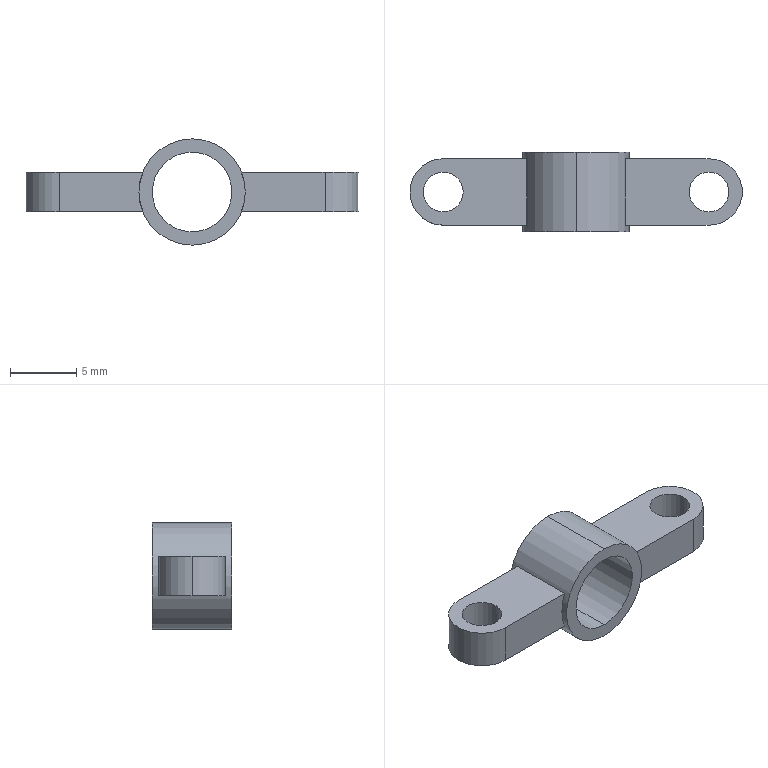Part | SolidWorks | features Extrusion 1, ICE 1 | 1 solid | 21 faces | box 25 x 6 x 8 mm | volume 331.315 mm3 | cylinder 11 | plane 10 | commonest cylinder face diameters 3 x4 5 x3 6 x2 8 x2
STEP:
#1=CARTESIAN_POINT('',(-11.5,3.,1.5));
#2=VERTEX_POINT('',#1);
#3=CARTESIAN_POINT('',(-8.5,3.,1.5));
#4=VERTEX_POINT('',#3);
#5=CARTESIAN_POINT('',(-10.,3.,1.5));
#6=DIRECTION('',(0.,0.,1.));
#7=DIRECTION('',(1.,0.,0.));
#8=AXIS2_PLACEMENT_3D('',#5,#6,#7);
#9=CIRCLE('',#8,1.5);
#10=EDGE_CURVE('',#2,#4,#9,.T.);
#11=ORIENTED_EDGE('',*,*,#10,.T.);
#12=CARTESIAN_POINT('',(-8.5,3.,-1.5));
#13=VERTEX_POINT('',#12);
#14=CARTESIAN_POINT('',(-8.5,3.,1.5));
#15=DIRECTION('',(0.,0.,-1.));
#16=VECTOR('',#15,1000.);
#17=LINE('',#14,#16);
#18=EDGE_CURVE('',#4,#13,#17,.T.);
#19=ORIENTED_EDGE('',*,*,#18,.T.);
#20=CARTESIAN_POINT('',(-11.5,3.,-1.5));
#21=VERTEX_POINT('',#20);
#22=CARTESIAN_POINT('',(-10.,3.,-1.5));
#23=DIRECTION('',(0.,0.,1.));
#24=DIRECTION('',(1.,0.,0.));
#25=AXIS2_PLACEMENT_3D('',#22,#23,#24);
#26=CIRCLE('',#25,1.5);
#27=EDGE_CURVE('',#21,#13,#26,.T.);
#28=ORIENTED_EDGE('',*,*,#27,.F.);
#29=CARTESIAN_POINT('',(-11.5,3.,1.5));
#30=DIRECTION('',(0.,0.,-1.));
#31=VECTOR('',#30,1000.);
#32=LINE('',#29,#31);
#33=EDGE_CURVE('',#2,#21,#32,.T.);
#34=ORIENTED_EDGE('',*,*,#33,.F.);
#35=EDGE_LOOP('',(#11,#19,#28,#34));
#36=FACE_OUTER_BOUND('',#35,.T.);
#37=CARTESIAN_POINT('',(-10.,3.,1.5));
#38=DIRECTION('',(0.,0.,-1.));
#39=DIRECTION('',(-1.,0.,0.));
#40=AXIS2_PLACEMENT_3D('',#37,#38,#39);
#41=CYLINDRICAL_SURFACE('',#40,1.5);
#42=ADVANCED_FACE('',(#36),#41,.F.);
#43=CARTESIAN_POINT('',(-12.5,3.,1.5));
#44=VERTEX_POINT('',#43);
#45=CARTESIAN_POINT('',(-10.,0.5,1.5));
#46=VERTEX_POINT('',#45);
#47=CARTESIAN_POINT('',(-10.,3.,1.5));
#48=DIRECTION('',(0.,0.,1.));
#49=DIRECTION('',(1.,0.,0.));
#50=AXIS2_PLACEMENT_3D('',#47,#48,#49);
#51=CIRCLE('',#50,2.5);
#52=EDGE_CURVE('',#44,#46,#51,.T.);
#53=ORIENTED_EDGE('',*,*,#52,.F.);
#54=CARTESIAN_POINT('',(-12.5,3.,-1.5));
#55=VERTEX_POINT('',#54);
#56=CARTESIAN_POINT('',(-12.5,3.,1.5));
#57=DIRECTION('',(0.,0.,-1.));
#58=VECTOR('',#57,1000.);
#59=LINE('',#56,#58);
#60=EDGE_CURVE('',#44,#55,#59,.T.);
#61=ORIENTED_EDGE('',*,*,#60,.T.);
#62=CARTESIAN_POINT('',(-10.,0.5,-1.5));
#63=VERTEX_POINT('',#62);
#64=CARTESIAN_POINT('',(-10.,3.,-1.5));
#65=DIRECTION('',(0.,0.,1.));
#66=DIRECTION('',(1.,0.,0.));
#67=AXIS2_PLACEMENT_3D('',#64,#65,#66);
#68=CIRCLE('',#67,2.5);
#69=EDGE_CURVE('',#55,#63,#68,.T.);
#70=ORIENTED_EDGE('',*,*,#69,.T.);
#71=CARTESIAN_POINT('',(-10.,0.5,1.5));
#72=DIRECTION('',(0.,0.,-1.));
#73=VECTOR('',#72,1000.);
#74=LINE('',#71,#73);
#75=EDGE_CURVE('',#46,#63,#74,.T.);
#76=ORIENTED_EDGE('',*,*,#75,.F.);
#77=EDGE_LOOP('',(#53,#61,#70,#76));
#78=FACE_OUTER_BOUND('',#77,.T.);
#79=CARTESIAN_POINT('',(-10.,3.,1.5));
#80=DIRECTION('',(0.,0.,-1.));
#81=DIRECTION('',(-1.,0.,0.));
#82=AXIS2_PLACEMENT_3D('',#79,#80,#81);
#83=CYLINDRICAL_SURFACE('',#82,2.5);
#84=ADVANCED_FACE('',(#78),#83,.T.);
#85=CARTESIAN_POINT('',(11.5,3.,1.5));
#86=VERTEX_POINT('',#85);
#87=CARTESIAN_POINT('',(8.5,3.,1.5));
#88=VERTEX_POINT('',#87);
#89=CARTESIAN_POINT('',(10.,3.,1.5));
#90=DIRECTION('',(0.,0.,-1.));
#91=DIRECTION('',(1.,0.,0.));
#92=AXIS2_PLACEMENT_3D('',#89,#90,#91);
#93=CIRCLE('',#92,1.5);
#94=EDGE_CURVE('',#86,#88,#93,.T.);
#95=ORIENTED_EDGE('',*,*,#94,.F.);
#96=CARTESIAN_POINT('',(11.5,3.,-1.5));
#97=VERTEX_POINT('',#96);
#98=CARTESIAN_POINT('',(11.5,3.,1.5));
#99=DIRECTION('',(0.,0.,-1.));
#100=VECTOR('',#99,1000.);
#101=LINE('',#98,#100);
#102=EDGE_CURVE('',#86,#97,#101,.T.);
#103=ORIENTED_EDGE('',*,*,#102,.T.);
#104=CARTESIAN_POINT('',(8.5,3.,-1.5));
#105=VERTEX_POINT('',#104);
#106=CARTESIAN_POINT('',(10.,3.,-1.5));
#107=DIRECTION('',(0.,0.,-1.));
#108=DIRECTION('',(1.,0.,0.));
#109=AXIS2_PLACEMENT_3D('',#106,#107,#108);
#110=CIRCLE('',#109,1.5);
#111=EDGE_CURVE('',#97,#105,#110,.T.);
#112=ORIENTED_EDGE('',*,*,#111,.T.);
#113=CARTESIAN_POINT('',(8.5,3.,1.5));
#114=DIRECTION('',(0.,0.,-1.));
#115=VECTOR('',#114,1000.);
#116=LINE('',#113,#115);
#117=EDGE_CURVE('',#88,#105,#116,.T.);
#118=ORIENTED_EDGE('',*,*,#117,.F.);
#119=EDGE_LOOP('',(#95,#103,#112,#118));
#120=FACE_OUTER_BOUND('',#119,.T.);
#121=CARTESIAN_POINT('',(10.,3.,1.5));
#122=DIRECTION('',(0.,0.,-1.));
#123=DIRECTION('',(-1.,0.,0.));
#124=AXIS2_PLACEMENT_3D('',#121,#122,#123);
#125=CYLINDRICAL_SURFACE('',#124,1.5);
#126=ADVANCED_FACE('',(#120),#125,.F.);
#127=CARTESIAN_POINT('',(0.,6.,-3.));
#128=VERTEX_POINT('',#127);
#129=CARTESIAN_POINT('',(0.,6.,3.));
#130=VERTEX_POINT('',#129);
#131=CARTESIAN_POINT('',(0.,6.,0.));
#132=DIRECTION('',(0.,1.,0.));
#133=DIRECTION('',(0.,0.,1.));
#134=AXIS2_PLACEMENT_3D('',#131,#132,#133);
#135=CIRCLE('',#134,3.);
#136=EDGE_CURVE('',#128,#130,#135,.T.);
#137=ORIENTED_EDGE('',*,*,#136,.T.);
#138=CARTESIAN_POINT('',(0.,0.,3.));
#139=VERTEX_POINT('',#138);
#140=CARTESIAN_POINT('',(0.,6.,3.));
#141=DIRECTION('',(0.,-1.,0.));
#142=VECTOR('',#141,1000.);
#143=LINE('',#140,#142);
#144=EDGE_CURVE('',#130,#139,#143,.T.);
#145=ORIENTED_EDGE('',*,*,#144,.T.);
#146=CARTESIAN_POINT('',(0.,0.,-3.));
#147=VERTEX_POINT('',#146);
#148=CARTESIAN_POINT('',(0.,0.,0.));
#149=DIRECTION('',(0.,1.,0.));
#150=DIRECTION('',(0.,0.,1.));
#151=AXIS2_PLACEMENT_3D('',#148,#149,#150);
#152=CIRCLE('',#151,3.);
#153=EDGE_CURVE('',#147,#139,#152,.T.);
#154=ORIENTED_EDGE('',*,*,#153,.F.);
#155=CARTESIAN_POINT('',(0.,6.,-3.));
#156=DIRECTION('',(0.,-1.,0.));
#157=VECTOR('',#156,1000.);
#158=LINE('',#155,#157);
#159=EDGE_CURVE('',#128,#147,#158,.T.);
#160=ORIENTED_EDGE('',*,*,#159,.F.);
#161=EDGE_LOOP('',(#137,#145,#154,#160));
#162=FACE_OUTER_BOUND('',#161,.T.);
#163=CARTESIAN_POINT('',(0.,6.,0.));
#164=DIRECTION('',(0.,-1.,0.));
#165=DIRECTION('',(0.,0.,-1.));
#166=AXIS2_PLACEMENT_3D('',#163,#164,#165);
#167=CYLINDRICAL_SURFACE('',#166,3.);
#168=ADVANCED_FACE('',(#162),#167,.F.);
#169=CARTESIAN_POINT('',(3.708,0.5,1.5));
#170=VERTEX_POINT('',#169);
#171=CARTESIAN_POINT('',(3.708,0.5,-1.5));
#172=VERTEX_POINT('',#171);
#173=CARTESIAN_POINT('',(0.,0.5,0.));
#174=DIRECTION('',(0.,1.,0.));
#175=DIRECTION('',(-1.,0.,0.));
#176=AXIS2_PLACEMENT_3D('',#173,#174,#175);
#177=CIRCLE('',#176,4.);
#178=EDGE_CURVE('',#170,#172,#177,.T.);
#179=ORIENTED_EDGE('',*,*,#178,.F.);
#180=CARTESIAN_POINT('',(3.708,5.5,1.5));
#181=VERTEX_POINT('',#180);
#182=CARTESIAN_POINT('',(3.708,6.,1.5));
#183=DIRECTION('',(0.,1.,0.));
#184=VECTOR('',#183,1000.);
#185=LINE('',#182,#184);
#186=EDGE_CURVE('',#170,#181,#185,.T.);
#187=ORIENTED_EDGE('',*,*,#186,.T.);
#188=CARTESIAN_POINT('',(3.708,5.5,-1.5));
#189=VERTEX_POINT('',#188);
#190=CARTESIAN_POINT('',(0.,5.5,0.));
#191=DIRECTION('',(0.,-1.,0.));
#192=DIRECTION('',(0.,0.,-1.));
#193=AXIS2_PLACEMENT_3D('',#190,#191,#192);
#194=CIRCLE('',#193,4.);
#195=EDGE_CURVE('',#189,#181,#194,.T.);
#196=ORIENTED_EDGE('',*,*,#195,.F.);
#197=CARTESIAN_POINT('',(3.708,6.,-1.5));
#198=DIRECTION('',(0.,1.,0.));
#199=VECTOR('',#198,1000.);
#200=LINE('',#197,#199);
#201=EDGE_CURVE('',#172,#189,#200,.T.);
#202=ORIENTED_EDGE('',*,*,#201,.F.);
#203=EDGE_LOOP('',(#179,#187,#196,#202));
#204=FACE_BOUND('',#203,.T.);
#205=CARTESIAN_POINT('',(0.,6.,4.));
#206=VERTEX_POINT('',#205);
#207=CARTESIAN_POINT('',(0.,6.,-4.));
#208=VERTEX_POINT('',#207);
#209=CARTESIAN_POINT('',(0.,6.,0.));
#210=DIRECTION('',(0.,1.,0.));
#211=DIRECTION('',(0.,0.,1.));
#212=AXIS2_PLACEMENT_3D('',#209,#210,#211);
#213=CIRCLE('',#212,4.);
#214=EDGE_CURVE('',#206,#208,#213,.T.);
#215=ORIENTED_EDGE('',*,*,#214,.F.);
#216=CARTESIAN_POINT('',(0.,0.,4.));
#217=VERTEX_POINT('',#216);
#218=CARTESIAN_POINT('',(0.,6.,4.));
#219=DIRECTION('',(0.,-1.,0.));
#220=VECTOR('',#219,1000.);
#221=LINE('',#218,#220);
#222=EDGE_CURVE('',#206,#217,#221,.T.);
#223=ORIENTED_EDGE('',*,*,#222,.T.);
#224=CARTESIAN_POINT('',(0.,0.,-4.));
#225=VERTEX_POINT('',#224);
#226=CARTESIAN_POINT('',(0.,0.,0.));
#227=DIRECTION('',(0.,1.,0.));
#228=DIRECTION('',(0.,0.,1.));
#229=AXIS2_PLACEMENT_3D('',#226,#227,#228);
#230=CIRCLE('',#229,4.);
#231=EDGE_CURVE('',#217,#225,#230,.T.);
#232=ORIENTED_EDGE('',*,*,#231,.T.);
#233=CARTESIAN_POINT('',(0.,6.,-4.));
#234=DIRECTION('',(0.,-1.,0.));
#235=VECTOR('',#234,1000.);
#236=LINE('',#233,#235);
#237=EDGE_CURVE('',#208,#225,#236,.T.);
#238=ORIENTED_EDGE('',*,*,#237,.F.);
#239=EDGE_LOOP('',(#215,#223,#232,#238));
#240=FACE_OUTER_BOUND('',#239,.T.);
#241=CARTESIAN_POINT('',(0.,6.,0.));
#242=DIRECTION('',(0.,-1.,0.));
#243=DIRECTION('',(0.,0.,-1.));
#244=AXIS2_PLACEMENT_3D('',#241,#242,#243);
#245=CYLINDRICAL_SURFACE('',#244,4.);
#246=ADVANCED_FACE('',(#204,#240),#245,.T.);
#247=CARTESIAN_POINT('',(0.,6.,0.));
#248=DIRECTION('',(0.,1.,0.));
#249=DIRECTION('',(0.,0.,1.));
#250=AXIS2_PLACEMENT_3D('',#247,#248,#249);
#251=CIRCLE('',#250,4.);
#252=EDGE_CURVE('',#208,#206,#251,.T.);
#253=ORIENTED_EDGE('',*,*,#252,.T.);
#254=ORIENTED_EDGE('',*,*,#214,.T.);
#255=EDGE_LOOP('',(#253,#254));
#256=FACE_OUTER_BOUND('',#255,.T.);
#257=ORIENTED_EDGE('',*,*,#136,.F.);
#258=CARTESIAN_POINT('',(0.,6.,0.));
#259=DIRECTION('',(0.,1.,0.));
#260=DIRECTION('',(0.,0.,1.));
#261=AXIS2_PLACEMENT_3D('',#258,#259,#260);
#262=CIRCLE('',#261,3.);
#263=EDGE_CURVE('',#130,#128,#262,.T.);
#264=ORIENTED_EDGE('',*,*,#263,.F.);
#265=EDGE_LOOP('',(#257,#264));
#266=FACE_BOUND('',#265,.T.);
#267=CARTESIAN_POINT('',(0.,6.,0.));
#268=DIRECTION('',(0.,1.,0.));
#269=DIRECTION('',(0.,0.,1.));
#270=AXIS2_PLACEMENT_3D('',#267,#268,#269);
#271=PLANE('',#270);
#272=ADVANCED_FACE('',(#256,#266),#271,.T.);
#273=CARTESIAN_POINT('',(0.,0.,0.));
#274=DIRECTION('',(0.,1.,0.));
#275=DIRECTION('',(0.,0.,1.));
#276=AXIS2_PLACEMENT_3D('',#273,#274,#275);
#277=CIRCLE('',#276,4.);
#278=EDGE_CURVE('',#225,#217,#277,.T.);
#279=ORIENTED_EDGE('',*,*,#278,.F.);
#280=ORIENTED_EDGE('',*,*,#231,.F.);
#281=EDGE_LOOP('',(#279,#280));
#282=FACE_OUTER_BOUND('',#281,.T.);
#283=ORIENTED_EDGE('',*,*,#153,.T.);
#284=CARTESIAN_POINT('',(0.,0.,0.));
#285=DIRECTION('',(0.,1.,0.));
#286=DIRECTION('',(0.,0.,1.));
#287=AXIS2_PLACEMENT_3D('',#284,#285,#286);
#288=CIRCLE('',#287,3.);
#289=EDGE_CURVE('',#139,#147,#288,.T.);
#290=ORIENTED_EDGE('',*,*,#289,.T.);
#291=EDGE_LOOP('',(#283,#290));
#292=FACE_BOUND('',#291,.T.);
#293=CARTESIAN_POINT('',(0.,0.,0.));
#294=DIRECTION('',(0.,1.,0.));
#295=DIRECTION('',(0.,0.,1.));
#296=AXIS2_PLACEMENT_3D('',#293,#294,#295);
#297=PLANE('',#296);
#298=ADVANCED_FACE('',(#282,#292),#297,.F.);
#299=ORIENTED_EDGE('',*,*,#222,.F.);
#300=ORIENTED_EDGE('',*,*,#252,.F.);
#301=ORIENTED_EDGE('',*,*,#237,.T.);
#302=ORIENTED_EDGE('',*,*,#278,.T.);
#303=EDGE_LOOP('',(#299,#300,#301,#302));
#304=FACE_OUTER_BOUND('',#303,.T.);
#305=CARTESIAN_POINT('',(-3.708,5.5,-1.5));
#306=VERTEX_POINT('',#305);
#307=CARTESIAN_POINT('',(-3.708,5.5,1.5));
#308=VERTEX_POINT('',#307);
#309=CARTESIAN_POINT('',(0.,5.5,0.));
#310=DIRECTION('',(0.,1.,0.));
#311=DIRECTION('',(0.,0.,1.));
#312=AXIS2_PLACEMENT_3D('',#309,#310,#311);
#313=CIRCLE('',#312,4.);
#314=EDGE_CURVE('',#306,#308,#313,.T.);
#315=ORIENTED_EDGE('',*,*,#314,.T.);
#316=CARTESIAN_POINT('',(-3.708,0.5,1.5));
#317=VERTEX_POINT('',#316);
#318=CARTESIAN_POINT('',(-3.708,6.,1.5));
#319=DIRECTION('',(0.,-1.,0.));
#320=VECTOR('',#319,1000.);
#321=LINE('',#318,#320);
#322=EDGE_CURVE('',#308,#317,#321,.T.);
#323=ORIENTED_EDGE('',*,*,#322,.T.);
#324=CARTESIAN_POINT('',(-3.708,0.5,-1.5));
#325=VERTEX_POINT('',#324);
#326=CARTESIAN_POINT('',(0.,0.5,0.));
#327=DIRECTION('',(0.,-1.,0.));
#328=DIRECTION('',(1.,0.,0.));
#329=AXIS2_PLACEMENT_3D('',#326,#327,#328);
#330=CIRCLE('',#329,4.);
#331=EDGE_CURVE('',#317,#325,#330,.T.);
#332=ORIENTED_EDGE('',*,*,#331,.T.);
#333=CARTESIAN_POINT('',(-3.708,6.,-1.5));
#334=DIRECTION('',(0.,-1.,0.));
#335=VECTOR('',#334,1000.);
#336=LINE('',#333,#335);
#337=EDGE_CURVE('',#306,#325,#336,.T.);
#338=ORIENTED_EDGE('',*,*,#337,.F.);
#339=EDGE_LOOP('',(#315,#323,#332,#338));
#340=FACE_BOUND('',#339,.T.);
#341=CARTESIAN_POINT('',(0.,6.,0.));
#342=DIRECTION('',(0.,-1.,0.));
#343=DIRECTION('',(0.,0.,-1.));
#344=AXIS2_PLACEMENT_3D('',#341,#342,#343);
#345=CYLINDRICAL_SURFACE('',#344,4.);
#346=ADVANCED_FACE('',(#304,#340),#345,.T.);
#347=ORIENTED_EDGE('',*,*,#144,.F.);
#348=ORIENTED_EDGE('',*,*,#263,.T.);
#349=ORIENTED_EDGE('',*,*,#159,.T.);
#350=ORIENTED_EDGE('',*,*,#289,.F.);
#351=EDGE_LOOP('',(#347,#348,#349,#350));
#352=FACE_OUTER_BOUND('',#351,.T.);
#353=CARTESIAN_POINT('',(0.,6.,0.));
#354=DIRECTION('',(0.,-1.,0.));
#355=DIRECTION('',(0.,0.,-1.));
#356=AXIS2_PLACEMENT_3D('',#353,#354,#355);
#357=CYLINDRICAL_SURFACE('',#356,3.);
#358=ADVANCED_FACE('',(#352),#357,.F.);
#359=CARTESIAN_POINT('',(10.,3.,1.5));
#360=DIRECTION('',(0.,0.,-1.));
#361=DIRECTION('',(1.,0.,0.));
#362=AXIS2_PLACEMENT_3D('',#359,#360,#361);
#363=CIRCLE('',#362,1.5);
#364=EDGE_CURVE('',#88,#86,#363,.T.);
#365=ORIENTED_EDGE('',*,*,#364,.T.);
#366=ORIENTED_EDGE('',*,*,#94,.T.);
#367=EDGE_LOOP('',(#365,#366));
#368=FACE_BOUND('',#367,.T.);
#369=ORIENTED_EDGE('',*,*,#186,.F.);
#370=CARTESIAN_POINT('',(10.,0.5,1.5));
#371=VERTEX_POINT('',#370);
#372=CARTESIAN_POINT('',(0.,0.5,1.5));
#373=DIRECTION('',(1.,0.,0.));
#374=VECTOR('',#373,1000.);
#375=LINE('',#372,#374);
#376=EDGE_CURVE('',#170,#371,#375,.T.);
#377=ORIENTED_EDGE('',*,*,#376,.T.);
#378=CARTESIAN_POINT('',(10.,5.5,1.5));
#379=VERTEX_POINT('',#378);
#380=CARTESIAN_POINT('',(10.,3.,1.5));
#381=DIRECTION('',(0.,0.,-1.));
#382=DIRECTION('',(1.,0.,0.));
#383=AXIS2_PLACEMENT_3D('',#380,#381,#382);
#384=CIRCLE('',#383,2.5);
#385=EDGE_CURVE('',#379,#371,#384,.T.);
#386=ORIENTED_EDGE('',*,*,#385,.F.);
#387=CARTESIAN_POINT('',(0.,5.5,1.5));
#388=DIRECTION('',(-1.,0.,0.));
#389=VECTOR('',#388,1000.);
#390=LINE('',#387,#389);
#391=EDGE_CURVE('',#379,#181,#390,.T.);
#392=ORIENTED_EDGE('',*,*,#391,.T.);
#393=EDGE_LOOP('',(#369,#377,#386,#392));
#394=FACE_OUTER_BOUND('',#393,.T.);
#395=CARTESIAN_POINT('',(0.,0.,1.5));
#396=DIRECTION('',(0.,0.,1.));
#397=DIRECTION('',(1.,0.,0.));
#398=AXIS2_PLACEMENT_3D('',#395,#396,#397);
#399=PLANE('',#398);
#400=ADVANCED_FACE('',(#368,#394),#399,.T.);
#401=CARTESIAN_POINT('',(10.,3.,-1.5));
#402=DIRECTION('',(0.,0.,-1.));
#403=DIRECTION('',(1.,0.,0.));
#404=AXIS2_PLACEMENT_3D('',#401,#402,#403);
#405=CIRCLE('',#404,1.5);
#406=EDGE_CURVE('',#105,#97,#405,.T.);
#407=ORIENTED_EDGE('',*,*,#406,.F.);
#408=ORIENTED_EDGE('',*,*,#111,.F.);
#409=EDGE_LOOP('',(#407,#408));
#410=FACE_BOUND('',#409,.T.);
#411=CARTESIAN_POINT('',(10.,0.5,-1.5));
#412=VERTEX_POINT('',#411);
#413=CARTESIAN_POINT('',(0.,0.5,-1.5));
#414=DIRECTION('',(1.,0.,0.));
#415=VECTOR('',#414,1000.);
#416=LINE('',#413,#415);
#417=EDGE_CURVE('',#172,#412,#416,.T.);
#418=ORIENTED_EDGE('',*,*,#417,.F.);
#419=ORIENTED_EDGE('',*,*,#201,.T.);
#420=CARTESIAN_POINT('',(10.,5.5,-1.5));
#421=VERTEX_POINT('',#420);
#422=CARTESIAN_POINT('',(0.,5.5,-1.5));
#423=DIRECTION('',(-1.,0.,0.));
#424=VECTOR('',#423,1000.);
#425=LINE('',#422,#424);
#426=EDGE_CURVE('',#421,#189,#425,.T.);
#427=ORIENTED_EDGE('',*,*,#426,.F.);
#428=CARTESIAN_POINT('',(10.,3.,-1.5));
#429=DIRECTION('',(0.,0.,-1.));
#430=DIRECTION('',(1.,0.,0.));
#431=AXIS2_PLACEMENT_3D('',#428,#429,#430);
#432=CIRCLE('',#431,2.5);
#433=EDGE_CURVE('',#421,#412,#432,.T.);
#434=ORIENTED_EDGE('',*,*,#433,.T.);
#435=EDGE_LOOP('',(#418,#419,#427,#434));
#436=FACE_OUTER_BOUND('',#435,.T.);
#437=CARTESIAN_POINT('',(0.,0.,-1.5));
#438=DIRECTION('',(0.,0.,1.));
#439=DIRECTION('',(1.,0.,0.));
#440=AXIS2_PLACEMENT_3D('',#437,#438,#439);
#441=PLANE('',#440);
#442=ADVANCED_FACE('',(#410,#436),#441,.F.);
#443=ORIENTED_EDGE('',*,*,#376,.F.);
#444=ORIENTED_EDGE('',*,*,#178,.T.);
#445=ORIENTED_EDGE('',*,*,#417,.T.);
#446=CARTESIAN_POINT('',(10.,0.5,1.5));
#447=DIRECTION('',(0.,0.,-1.));
#448=VECTOR('',#447,1000.);
#449=LINE('',#446,#448);
#450=EDGE_CURVE('',#371,#412,#449,.T.);
#451=ORIENTED_EDGE('',*,*,#450,.F.);
#452=EDGE_LOOP('',(#443,#444,#445,#451));
#453=FACE_OUTER_BOUND('',#452,.T.);
#454=CARTESIAN_POINT('',(0.,0.5,1.5));
#455=DIRECTION('',(0.,1.,0.));
#456=DIRECTION('',(-1.,0.,0.));
#457=AXIS2_PLACEMENT_3D('',#454,#455,#456);
#458=PLANE('',#457);
#459=ADVANCED_FACE('',(#453),#458,.F.);
#460=ORIENTED_EDGE('',*,*,#433,.F.);
#461=CARTESIAN_POINT('',(10.,5.5,1.5));
#462=DIRECTION('',(0.,0.,-1.));
#463=VECTOR('',#462,1000.);
#464=LINE('',#461,#463);
#465=EDGE_CURVE('',#379,#421,#464,.T.);
#466=ORIENTED_EDGE('',*,*,#465,.F.);
#467=ORIENTED_EDGE('',*,*,#385,.T.);
#468=ORIENTED_EDGE('',*,*,#450,.T.);
#469=EDGE_LOOP('',(#460,#466,#467,#468));
#470=FACE_OUTER_BOUND('',#469,.T.);
#471=CARTESIAN_POINT('',(10.,3.,1.5));
#472=DIRECTION('',(0.,0.,-1.));
#473=DIRECTION('',(-1.,0.,0.));
#474=AXIS2_PLACEMENT_3D('',#471,#472,#473);
#475=CYLINDRICAL_SURFACE('',#474,2.5);
#476=ADVANCED_FACE('',(#470),#475,.T.);
#477=ORIENTED_EDGE('',*,*,#426,.T.);
#478=ORIENTED_EDGE('',*,*,#195,.T.);
#479=ORIENTED_EDGE('',*,*,#391,.F.);
#480=ORIENTED_EDGE('',*,*,#465,.T.);
#481=EDGE_LOOP('',(#477,#478,#479,#480));
#482=FACE_OUTER_BOUND('',#481,.T.);
#483=CARTESIAN_POINT('',(0.,5.5,1.5));
#484=DIRECTION('',(0.,-1.,0.));
#485=DIRECTION('',(0.,0.,-1.));
#486=AXIS2_PLACEMENT_3D('',#483,#484,#485);
#487=PLANE('',#486);
#488=ADVANCED_FACE('',(#482),#487,.F.);
#489=ORIENTED_EDGE('',*,*,#102,.F.);
#490=ORIENTED_EDGE('',*,*,#364,.F.);
#491=ORIENTED_EDGE('',*,*,#117,.T.);
#492=ORIENTED_EDGE('',*,*,#406,.T.);
#493=EDGE_LOOP('',(#489,#490,#491,#492));
#494=FACE_OUTER_BOUND('',#493,.T.);
#495=CARTESIAN_POINT('',(10.,3.,1.5));
#496=DIRECTION('',(0.,0.,-1.));
#497=DIRECTION('',(-1.,0.,0.));
#498=AXIS2_PLACEMENT_3D('',#495,#496,#497);
#499=CYLINDRICAL_SURFACE('',#498,1.5);
#500=ADVANCED_FACE('',(#494),#499,.F.);
#501=ORIENTED_EDGE('',*,*,#10,.F.);
#502=CARTESIAN_POINT('',(-10.,3.,1.5));
#503=DIRECTION('',(0.,0.,1.));
#504=DIRECTION('',(1.,0.,0.));
#505=AXIS2_PLACEMENT_3D('',#502,#503,#504);
#506=CIRCLE('',#505,1.5);
#507=EDGE_CURVE('',#4,#2,#506,.T.);
#508=ORIENTED_EDGE('',*,*,#507,.F.);
#509=EDGE_LOOP('',(#501,#508));
#510=FACE_BOUND('',#509,.T.);
#511=ORIENTED_EDGE('',*,*,#322,.F.);
#512=CARTESIAN_POINT('',(-10.,5.5,1.5));
#513=VERTEX_POINT('',#512);
#514=CARTESIAN_POINT('',(0.,5.5,1.5));
#515=DIRECTION('',(1.,0.,0.));
#516=VECTOR('',#515,1000.);
#517=LINE('',#514,#516);
#518=EDGE_CURVE('',#513,#308,#517,.T.);
#519=ORIENTED_EDGE('',*,*,#518,.F.);
#520=CARTESIAN_POINT('',(-10.,3.,1.5));
#521=DIRECTION('',(0.,0.,1.));
#522=DIRECTION('',(1.,0.,0.));
#523=AXIS2_PLACEMENT_3D('',#520,#521,#522);
#524=CIRCLE('',#523,2.5);
#525=EDGE_CURVE('',#513,#44,#524,.T.);
#526=ORIENTED_EDGE('',*,*,#525,.T.);
#527=ORIENTED_EDGE('',*,*,#52,.T.);
#528=CARTESIAN_POINT('',(0.,0.5,1.5));
#529=DIRECTION('',(-1.,0.,0.));
#530=VECTOR('',#529,1000.);
#531=LINE('',#528,#530);
#532=EDGE_CURVE('',#317,#46,#531,.T.);
#533=ORIENTED_EDGE('',*,*,#532,.F.);
#534=EDGE_LOOP('',(#511,#519,#526,#527,#533));
#535=FACE_OUTER_BOUND('',#534,.T.);
#536=CARTESIAN_POINT('',(0.,0.,1.5));
#537=DIRECTION('',(0.,0.,1.));
#538=DIRECTION('',(1.,0.,0.));
#539=AXIS2_PLACEMENT_3D('',#536,#537,#538);
#540=PLANE('',#539);
#541=ADVANCED_FACE('',(#510,#535),#540,.T.);
#542=ORIENTED_EDGE('',*,*,#27,.T.);
#543=CARTESIAN_POINT('',(-10.,3.,-1.5));
#544=DIRECTION('',(0.,0.,1.));
#545=DIRECTION('',(1.,0.,0.));
#546=AXIS2_PLACEMENT_3D('',#543,#544,#545);
#547=CIRCLE('',#546,1.5);
#548=EDGE_CURVE('',#13,#21,#547,.T.);
#549=ORIENTED_EDGE('',*,*,#548,.T.);
#550=EDGE_LOOP('',(#542,#549));
#551=FACE_BOUND('',#550,.T.);
#552=CARTESIAN_POINT('',(-10.,5.5,-1.5));
#553=VERTEX_POINT('',#552);
#554=CARTESIAN_POINT('',(0.,5.5,-1.5));
#555=DIRECTION('',(1.,0.,0.));
#556=VECTOR('',#555,1000.);
#557=LINE('',#554,#556);
#558=EDGE_CURVE('',#553,#306,#557,.T.);
#559=ORIENTED_EDGE('',*,*,#558,.T.);
#560=ORIENTED_EDGE('',*,*,#337,.T.);
#561=CARTESIAN_POINT('',(0.,0.5,-1.5));
#562=DIRECTION('',(-1.,0.,0.));
#563=VECTOR('',#562,1000.);
#564=LINE('',#561,#563);
#565=EDGE_CURVE('',#325,#63,#564,.T.);
#566=ORIENTED_EDGE('',*,*,#565,.T.);
#567=ORIENTED_EDGE('',*,*,#69,.F.);
#568=CARTESIAN_POINT('',(-10.,3.,-1.5));
#569=DIRECTION('',(0.,0.,1.));
#570=DIRECTION('',(1.,0.,0.));
#571=AXIS2_PLACEMENT_3D('',#568,#569,#570);
#572=CIRCLE('',#571,2.5);
#573=EDGE_CURVE('',#553,#55,#572,.T.);
#574=ORIENTED_EDGE('',*,*,#573,.F.);
#575=EDGE_LOOP('',(#559,#560,#566,#567,#574));
#576=FACE_OUTER_BOUND('',#575,.T.);
#577=CARTESIAN_POINT('',(0.,0.,-1.5));
#578=DIRECTION('',(0.,0.,1.));
#579=DIRECTION('',(1.,0.,0.));
#580=AXIS2_PLACEMENT_3D('',#577,#578,#579);
#581=PLANE('',#580);
#582=ADVANCED_FACE('',(#551,#576),#581,.F.);
#583=ORIENTED_EDGE('',*,*,#314,.F.);
#584=ORIENTED_EDGE('',*,*,#558,.F.);
#585=CARTESIAN_POINT('',(-10.,5.5,1.5));
#586=DIRECTION('',(0.,0.,-1.));
#587=VECTOR('',#586,1000.);
#588=LINE('',#585,#587);
#589=EDGE_CURVE('',#513,#553,#588,.T.);
#590=ORIENTED_EDGE('',*,*,#589,.F.);
#591=ORIENTED_EDGE('',*,*,#518,.T.);
#592=EDGE_LOOP('',(#583,#584,#590,#591));
#593=FACE_OUTER_BOUND('',#592,.T.);
#594=CARTESIAN_POINT('',(0.,5.5,1.5));
#595=DIRECTION('',(0.,1.,0.));
#596=DIRECTION('',(0.,0.,1.));
#597=AXIS2_PLACEMENT_3D('',#594,#595,#596);
#598=PLANE('',#597);
#599=ADVANCED_FACE('',(#593),#598,.T.);
#600=ORIENTED_EDGE('',*,*,#60,.F.);
#601=ORIENTED_EDGE('',*,*,#525,.F.);
#602=ORIENTED_EDGE('',*,*,#589,.T.);
#603=ORIENTED_EDGE('',*,*,#573,.T.);
#604=EDGE_LOOP('',(#600,#601,#602,#603));
#605=FACE_OUTER_BOUND('',#604,.T.);
#606=CARTESIAN_POINT('',(-10.,3.,1.5));
#607=DIRECTION('',(0.,0.,-1.));
#608=DIRECTION('',(-1.,0.,0.));
#609=AXIS2_PLACEMENT_3D('',#606,#607,#608);
#610=CYLINDRICAL_SURFACE('',#609,2.5);
#611=ADVANCED_FACE('',(#605),#610,.T.);
#612=ORIENTED_EDGE('',*,*,#331,.F.);
#613=ORIENTED_EDGE('',*,*,#532,.T.);
#614=ORIENTED_EDGE('',*,*,#75,.T.);
#615=ORIENTED_EDGE('',*,*,#565,.F.);
#616=EDGE_LOOP('',(#612,#613,#614,#615));
#617=FACE_OUTER_BOUND('',#616,.T.);
#618=CARTESIAN_POINT('',(0.,0.5,1.5));
#619=DIRECTION('',(0.,-1.,0.));
#620=DIRECTION('',(1.,0.,0.));
#621=AXIS2_PLACEMENT_3D('',#618,#619,#620);
#622=PLANE('',#621);
#623=ADVANCED_FACE('',(#617),#622,.T.);
#624=ORIENTED_EDGE('',*,*,#18,.F.);
#625=ORIENTED_EDGE('',*,*,#507,.T.);
#626=ORIENTED_EDGE('',*,*,#33,.T.);
#627=ORIENTED_EDGE('',*,*,#548,.F.);
#628=EDGE_LOOP('',(#624,#625,#626,#627));
#629=FACE_OUTER_BOUND('',#628,.T.);
#630=CARTESIAN_POINT('',(-10.,3.,1.5));
#631=DIRECTION('',(0.,0.,-1.));
#632=DIRECTION('',(-1.,0.,0.));
#633=AXIS2_PLACEMENT_3D('',#630,#631,#632);
#634=CYLINDRICAL_SURFACE('',#633,1.5);
#635=ADVANCED_FACE('',(#629),#634,.F.);
#636=CLOSED_SHELL('',(#42,#84,#126,#168,#246,#272,#298,#346,#358,#400,#442,#459,#476,#488,#500,#541,#582,#599,#611,#623,#635));
#637=MANIFOLD_SOLID_BREP('',#636);
#638=CARTESIAN_POINT('',(0.,0.,0.));
#639=DIRECTION('',(0.,0.,1.));
#640=DIRECTION('',(1.,0.,0.));
#641=AXIS2_PLACEMENT_3D('',#638,#639,#640);
#642=(LENGTH_UNIT()NAMED_UNIT(*)SI_UNIT(.MILLI.,.METRE.));
#643=UNCERTAINTY_MEASURE_WITH_UNIT(LENGTH_MEASURE(0.00001),#642,'','');
#644=(NAMED_UNIT(*)PLANE_ANGLE_UNIT()SI_UNIT($,.RADIAN.));
#645=(NAMED_UNIT(*)SI_UNIT($,.STERADIAN.)SOLID_ANGLE_UNIT());
#646=(GEOMETRIC_REPRESENTATION_CONTEXT(3)GLOBAL_UNCERTAINTY_ASSIGNED_CONTEXT((#643))GLOBAL_UNIT_ASSIGNED_CONTEXT((#642,#644,#645))REPRESENTATION_CONTEXT('',''));
#647=ADVANCED_BREP_SHAPE_REPRESENTATION('',(#637,#641),#646);